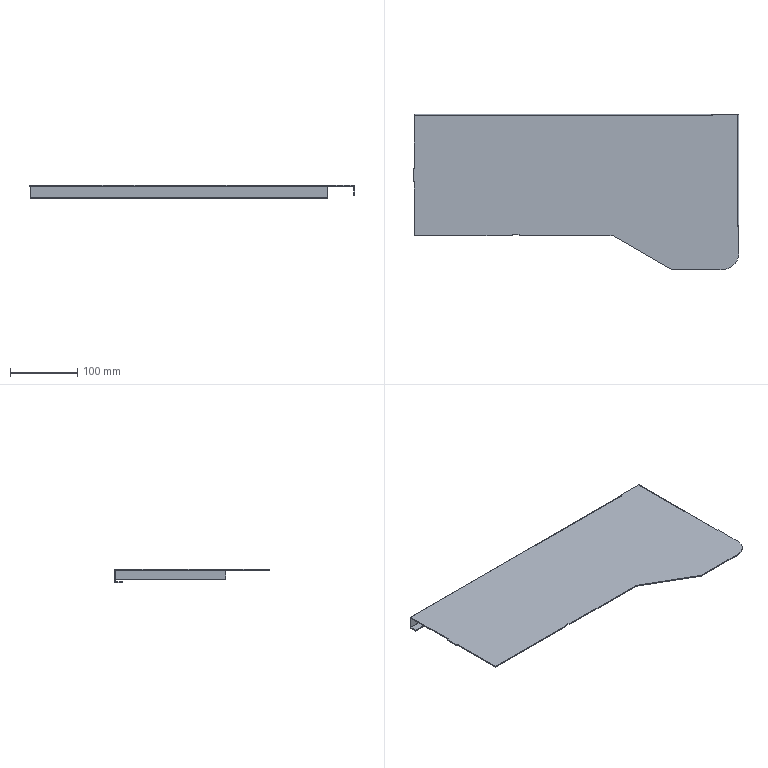Part | STEP file | FHD-021-001-H rack welded part H | 1 solid | 37 faces | box 483 x 230 x 20 mm | volume 162335 mm3 | plane 30 | cylinder 7 | commonest cylinder face diameters 0.4 x3 3.4 x3 50 x1